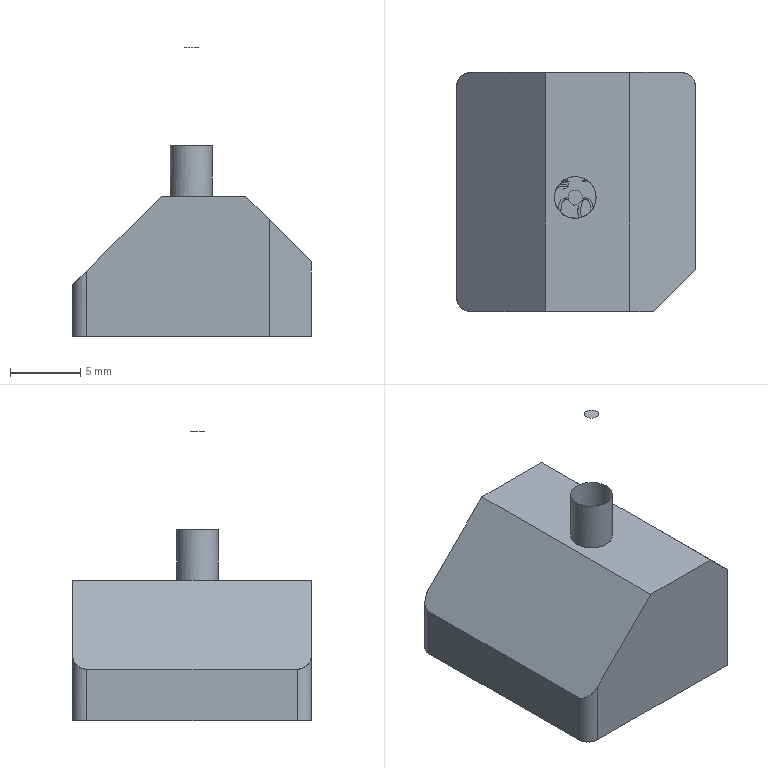NC program | PowerMill | posted with a generic post | part box 17 x 17 x 20.603 mm
Lines 3446 to 4194 of 69435:
N3543 M6
N3544 S8500 M03
N3545 G00 G90 X0.002 Y0.0
N3546 G43 Z11.803 H3
N3547
N3548 G05 P10000 R8
N3549 X2.657 Y10.5422
N3550 Z0.9529
N3551 G01 Z-0.2471 F360.0
N3552 X1.3839 Y5.4231 F600.0
N3553 X-4.833 Y-4.026
N3554 X-4.8208 Y-4.0426
N3555 G03 X-4.4372 Y-4.4965 I5.5114 J4.2692
N3556 G01 X-4.1788 Y-4.7566
N3557 X-3.8542 Y-5.0424
N3558 X-3.7339 Y-5.1386
N3559 X-3.531 Y-5.2892
N3560 X-3.2148 Y-5.4994
N3561 X-2.889 Y-5.6879
N3562 X-2.7291 Y-5.7704
N3563 X-2.5666 Y-5.8477
N3564 X-2.2505 Y-5.9835
N3565 X-2.023 Y-6.0667
N3566 X-1.726 Y-6.16
N3567 X-1.6019 Y-6.1971
N3568 X-1.4915 Y-6.2234
N3569 X4.7268 Y3.2278
N3570 G00 Z11.803
N3571 G05 P0
N3572 (---------------)
N3573 ( END TOOLPATH : 精公基准台01-平坦面平行-D10 )
N3574 (---------------)
N3575 ( START TOOLPATH : 精公基准台01-基准面偏置-D10 )
N3576 (---------------)
N3577 G00 X0.002 Y0.0 Z9.8029
N3578 G05 P10000 R8
N3579 X-11.42 Y14.0289
N3580 Z-9.6
N3581 G01 Z-10.8 F360.0
N3582 X-6.8515 Y11.3918 F600.0
N3583 X-6.3619 Y2.3433
N3584 X-6.2705 Y2.5538
N3585 X-6.1275 Y2.8375
N3586 X-5.9674 Y3.1213
N3587 X-5.7484 Y3.4657
N3588 X-5.5905 Y3.6888
N3589 X-5.3328 Y4.0166
N3590 X-5.1227 Y4.2563
N3591 X-4.9538 Y4.4336
N3592 X-4.7725 Y4.6109
N3593 X-4.5356 Y4.8238
N3594 X-4.2123 Y5.0848
N3595 X-3.993 Y5.2444
N3596 X-3.7737 Y5.3913
N3597 X-3.652 Y5.4675
N3598 X-3.3719 Y5.6304
N3599 X-3.0918 Y5.7767
N3600 X-2.6893 Y5.9588
N3601 X-2.5315 Y6.0219
N3602 X-2.2514 Y6.1232
N3603 X-1.9713 Y6.2112
N3604 X-1.6911 Y6.286
N3605 X-1.411 Y6.3486
N3606 X-1.1309 Y6.3989
N3607 X-0.8508 Y6.4376
N3608 X-0.5706 Y6.4644
N3609 X-0.2905 Y6.4797
N3610 X-0.0104 Y6.4838
N3611 X0.2697 Y6.4764
N3612 X0.5499 Y6.4574
N3613 X0.83 Y6.4271
N3614 X1.1101 Y6.385
N3615 X1.3903 Y6.3312
N3616 X1.6704 Y6.2649
N3617 X1.9505 Y6.186
N3618 X2.2306 Y6.0943
N3619 X2.5846 Y5.9588
N3620 X2.8278 Y5.8524
N3621 X3.071 Y5.7346
N3622 X3.3511 Y5.5835
N3623 X3.6687 Y5.3913
N3624 X3.9301 Y5.2148
N3625 X4.1915 Y5.0199
N3626 X4.4309 Y4.8238
N3627 X4.7518 Y4.5303
N3628 X5.0177 Y4.2563
N3629 X5.1677 Y4.0876
N3630 X5.312 Y3.914
N3631 X5.4857 Y3.6888
N3632 X5.6845 Y3.405
N3633 X5.8723 Y3.1049
N3634 X6.0267 Y2.8293
N3635 X6.1655 Y2.5538
N3636 X6.2927 Y2.27
N3637 X6.4325 Y1.9092
N3638 X6.5151 Y1.664
N3639 X6.5868 Y1.4188
N3640 X6.6582 Y1.135
N3641 X6.7167 Y0.8513
N3642 X6.7632 Y0.5675
N3643 X6.7974 Y0.2838
N3644 X6.8198 Y0.0
N3645 X6.8303 Y-0.2838
N3646 X6.8291 Y-0.5675
N3647 X6.8166 Y-0.8513
N3648 X6.7922 Y-1.135
N3649 X6.7556 Y-1.4188
N3650 X6.7072 Y-1.7025
N3651 X6.6462 Y-1.9863
N3652 X6.5728 Y-2.27
N3653 X6.4859 Y-2.5538
N3654 X6.4325 Y-2.7095
N3655 X6.2708 Y-3.1213
N3656 X6.141 Y-3.405
N3657 X5.9945 Y-3.6888
N3658 X5.8723 Y-3.9049
N3659 X5.6501 Y-4.2563
N3660 X5.4883 Y-4.4851
N3661 X5.312 Y-4.714
N3662 X5.222 Y-4.8238
N3663 X4.9987 Y-5.077
N3664 X4.6883 Y-5.3913
N3665 X4.4399 Y-5.6161
N3666 X4.1915 Y-5.8199
N3667 X4.0082 Y-5.9588
N3668 X3.6313 Y-6.2153
N3669 X3.3592 Y-6.379
N3670 X3.071 Y-6.5346
N3671 X2.7909 Y-6.6692
N3672 X2.5108 Y-6.7889
N3673 X2.2306 Y-6.8943
N3674 X1.9505 Y-6.986
N3675 X1.5541 Y-7.0938
N3676 X1.3903 Y-7.1312
N3677 X1.1101 Y-7.1849
N3678 X0.83 Y-7.227
N3679 X0.5499 Y-7.2576
N3680 X0.2697 Y-7.2764
N3681 X-0.0104 Y-7.2837
N3682 X-0.2905 Y-7.2797
N3683 X-0.5706 Y-7.2643
N3684 X-0.8508 Y-7.2376
N3685 X-1.1309 Y-7.1989
N3686 X-1.411 Y-7.1486
N3687 X-1.6588 Y-7.0938
N3688 X-1.9713 Y-7.0112
N3689 X-2.2514 Y-6.9233
N3690 X-2.5315 Y-6.8219
N3691 X-2.8116 Y-6.7068
N3692 X-3.0918 Y-6.5767
N3693 X-3.4219 Y-6.4028
N3694 X-3.652 Y-6.2674
N3695 X-3.8823 Y-6.1201
N3696 X-4.2123 Y-5.8848
N3697 X-4.4924 Y-5.6607
N3698 X-4.7725 Y-5.4109
N3699 X-5.0751 Y-5.1075
N3700 X-5.3267 Y-4.8238
N3701 X-5.5549 Y-4.5364
N3702 X-5.7549 Y-4.2563
N3703 X-5.893 Y-4.0426
N3704 X-6.0995 Y-3.6888
N3705 X-6.2457 Y-3.405
N3706 X-6.3756 Y-3.1213
N3707 X-6.4533 Y-2.9328
N3708 X-6.5906 Y-2.5538
N3709 X-6.6773 Y-2.27
N3710 X-6.7509 Y-1.9863
N3711 X-6.8119 Y-1.7025
N3712 X-6.8606 Y-1.4188
N3713 X-6.897 Y-1.135
N3714 X-6.9216 Y-0.8513
N3715 X-6.9337 Y-0.5675
N3716 X-6.935 Y-0.2838
N3717 X-6.9248 Y0.0
N3718 X-6.9022 Y0.2838
N3719 X-6.868 Y0.5675
N3720 X-6.8215 Y0.8513
N3721 X-6.7629 Y1.135
N3722 X-6.6918 Y1.4188
N3723 X-6.6073 Y1.7025
N3724 X-6.5093 Y1.9863
N3725 X-6.4533 Y2.1328
N3726 X-6.3619 Y2.3433
N3727 G00 Z9.8029
N3728 G05 P0
N3729 (---------------)
N3730 ( END TOOLPATH : 精公基准台01-基准面偏置-D10 )
N3731 (---------------)
N3732 ( START TOOLPATH : 精公基准台01-基准台侧光-D10 )
N3733 (---------------)
N3734 G00 X0.002 Y0.0 Z9.8029
N3735 G05 P10000 R8
N3736 X13.4804 Y-14.7765
N3737 Z-19.5
N3738 G01 Z-20.7 F360.0
N3739 G03 X9.9448 Y-11.241 I-1.7678 J1.7678 F600.0
N3740 G01 X9.1157 Y-12.0701
N3741 X9.1151 Y-12.0707
N3742 X9.1144 Y-12.0714
N3743 X8.9094 Y-12.2674
N3744 X8.908 Y-12.2686
N3745 X8.9066 Y-12.2699
N3746 X8.7687 Y-12.39
N3747 X8.7675 Y-12.3911
N3748 X8.7662 Y-12.3921
N3749 X8.588 Y-12.5349
N3750 X8.5863 Y-12.5362
N3751 X8.5846 Y-12.5375
N3752 X8.3433 Y-12.7108
N3753 X8.342 Y-12.7117
N3754 X8.3407 Y-12.7126
N3755 X8.2659 Y-12.762
N3756 X8.2644 Y-12.763
N3757 X8.2628 Y-12.764
N3758 X7.9467 Y-12.9528
N3759 X7.9448 Y-12.9539
N3760 X7.9429 Y-12.9549
N3761 X7.7951 Y-13.0328
N3762 X7.7939 Y-13.0334
N3763 X7.7926 Y-13.034
N3764 X7.6243 Y-13.1152
N3765 X7.6223 Y-13.1161
N3766 X7.6204 Y-13.117
N3767 X7.3042 Y-13.2494
N3768 X7.3018 Y-13.2503
N3769 X7.2993 Y-13.2512
N3770 X7.0005 Y-13.3538
N3771 X6.998 Y-13.3546
N3772 X6.9955 Y-13.3553
N3773 X6.662 Y-13.4457
N3774 X6.6594 Y-13.4463
N3775 X6.6568 Y-13.4469
N3776 X6.3406 Y-13.5102
N3777 X6.3381 Y-13.5107
N3778 X6.3356 Y-13.511
N3779 X6.0194 Y-13.5535
N3780 X6.0169 Y-13.5538
N3781 X6.0144 Y-13.554
N3782 X5.6982 Y-13.5762
N3783 X5.6959 Y-13.5763
N3784 X5.6935
N3785 X5.3774 Y-13.58
N3786 X5.3769
N3787 X5.3765
N3788 X-7.5855 Y-13.5793
N3789 X-7.5871 Y-13.5792
N3790 X-7.5887
N3791 X-7.9049 Y-13.5664
N3792 X-7.907 Y-13.5663
N3793 X-7.9091 Y-13.5661
N3794 X-8.2253 Y-13.5364
N3795 X-8.2274 Y-13.5361
N3796 X-8.2295 Y-13.5359
N3797 X-8.5456 Y-13.4891
N3798 X-8.5478 Y-13.4887
N3799 X-8.5498 Y-13.4883
N3800 X-8.866 Y-13.4242
N3801 X-8.8679 Y-13.4237
N3802 X-8.8699 Y-13.4233
N3803 X-9.1348 Y-13.3556
N3804 X-9.1369 Y-13.3551
N3805 X-9.139 Y-13.3544
N3806 X-9.5064 Y-13.2388
N3807 X-9.5087 Y-13.238
N3808 X-9.511 Y-13.2372
N3809 X-9.8271 Y-13.1162
N3810 X-9.8287 Y-13.1155
N3811 X-9.8304 Y-13.1148
N3812 X-10.0135 Y-13.0354
N3813 X-10.0146 Y-13.0349
N3814 X-10.0157 Y-13.0344
N3815 X-10.1487 Y-12.9719
N3816 X-10.1502 Y-12.9712
N3817 X-10.1517 Y-12.9704
N3818 X-10.4678 Y-12.8054
N3819 X-10.4694 Y-12.8046
N3820 X-10.4709 Y-12.8037
N3821 X-10.6239 Y-12.715
N3822 X-10.6249 Y-12.7144
N3823 X-10.6259 Y-12.7138
N3824 X-10.7892 Y-12.6124
N3825 X-10.7908 Y-12.6114
N3826 X-10.7924 Y-12.6103
N3827 X-11.1039 Y-12.3955
N3828 X-11.1061 Y-12.394
N3829 X-11.1081 Y-12.3924
N3830 X-11.4289 Y-12.1387
N3831 X-11.4302 Y-12.1376
N3832 X-11.4315 Y-12.1365
N3833 X-11.5039 Y-12.0741
N3834 X-11.505 Y-12.0732
N3835 X-11.506 Y-12.0722
N3836 X-11.7498 Y-11.8464
N3837 X-11.7509 Y-11.8454
N3838 X-11.752 Y-11.8443
N3839 X-11.8423 Y-11.754
N3840 X-11.8434 Y-11.7529
N3841 X-11.8444 Y-11.7518
N3842 X-12.0702 Y-11.508
N3843 X-12.0712 Y-11.507
N3844 X-12.0721 Y-11.5059
N3845 X-12.1346 Y-11.4335
N3846 X-12.1357 Y-11.4322
N3847 X-12.1367 Y-11.4309
N3848 X-12.3871 Y-11.1148
N3849 X-12.3887 Y-11.1127
N3850 X-12.3902 Y-11.1106
N3851 X-12.6085 Y-10.7944
N3852 X-12.6096 Y-10.7928
N3853 X-12.6106 Y-10.7912
N3854 X-12.7118 Y-10.6282
N3855 X-12.7124 Y-10.6272
N3856 X-12.713 Y-10.6262
N3857 X-12.8019 Y-10.4729
N3858 X-12.8028 Y-10.4714
N3859 X-12.8036 Y-10.4698
N3860 X-12.9687 Y-10.1537
N3861 X-12.9698 Y-10.1516
N3862 X-12.9708 Y-10.1494
N3863 X-13.1127 Y-9.8333
N3864 X-13.1136 Y-9.8312
N3865 X-13.1144 Y-9.8291
N3866 X-13.2354 Y-9.513
N3867 X-13.2361 Y-9.5109
N3868 X-13.2369 Y-9.5088
N3869 X-13.338 Y-9.1926
N3870 X-13.3387 Y-9.1905
N3871 X-13.3393 Y-9.1883
N3872 X-13.4213 Y-8.8722
N3873 X-13.4218 Y-8.8701
N3874 X-13.4223 Y-8.868
N3875 X-13.4867 Y-8.5519
N3876 X-13.4871 Y-8.5498
N3877 X-13.4875 Y-8.5476
N3878 X-13.5341 Y-8.2315
N3879 X-13.5344 Y-8.2294
N3880 X-13.5346 Y-8.2272
N3881 X-13.5642 Y-7.9111
N3882 X-13.5643 Y-7.909
N3883 X-13.5645 Y-7.907
N3884 X-13.5776 Y-7.5908
N3885 X-13.5777 Y-7.5892
N3886 Y-7.5875
N3887 Y0.0
N3888 Y7.5875
N3889 Y7.5892
N3890 X-13.5776 Y7.5908
N3891 X-13.5645 Y7.907
N3892 X-13.5643 Y7.909
N3893 X-13.5642 Y7.9111
N3894 X-13.5346 Y8.2272
N3895 X-13.5344 Y8.2294
N3896 X-13.5341 Y8.2315
N3897 X-13.4875 Y8.5476
N3898 X-13.4871 Y8.5498
N3899 X-13.4867 Y8.5519
N3900 X-13.4223 Y8.868
N3901 X-13.4219 Y8.8699
N3902 X-13.4214 Y8.8718
N3903 X-13.3536 Y9.1379
N3904 X-13.3531 Y9.14
N3905 X-13.3524 Y9.1422
N3906 X-13.237 Y9.5084
N3907 X-13.2362 Y9.5107
N3908 X-13.2354 Y9.513
N3909 X-13.1144 Y9.8291
N3910 X-13.1136 Y9.8312
N3911 X-13.1127 Y9.8333
N3912 X-12.9708 Y10.1494
N3913 X-12.9698 Y10.1516
N3914 X-12.9687 Y10.1537
N3915 X-12.8036 Y10.4698
N3916 X-12.8028 Y10.4714
N3917 X-12.8019 Y10.4729
N3918 X-12.713 Y10.6262
N3919 X-12.7124 Y10.6272
N3920 X-12.7118 Y10.6282
N3921 X-12.6106 Y10.7912
N3922 X-12.6096 Y10.7928
N3923 X-12.6085 Y10.7944
N3924 X-12.3935 Y11.106
N3925 X-12.392 Y11.1082
N3926 X-12.3904 Y11.1103
N3927 X-12.1367 Y11.4309
N3928 X-12.1357 Y11.4322
N3929 X-12.1346 Y11.4335
N3930 X-12.0721 Y11.5059
N3931 X-12.0712 Y11.507
N3932 X-12.0702 Y11.508
N3933 X-11.8444 Y11.7518
N3934 X-11.8434 Y11.7529
N3935 X-11.8423 Y11.754
N3936 X-11.752 Y11.8443
N3937 X-11.7509 Y11.8454
N3938 X-11.7498 Y11.8464
N3939 X-11.506 Y12.0722
N3940 X-11.505 Y12.0732
N3941 X-11.5039 Y12.0741
N3942 X-11.4315 Y12.1365
N3943 X-11.4302 Y12.1376
N3944 X-11.4289 Y12.1387
N3945 X-11.1128 Y12.389
N3946 X-11.1107 Y12.3906
N3947 X-11.1085 Y12.3921
N3948 X-10.7924 Y12.6103
N3949 X-10.7908 Y12.6114
N3950 X-10.7892 Y12.6124
N3951 X-10.6259 Y12.7138
N3952 X-10.6249 Y12.7144
N3953 X-10.6239 Y12.715
N3954 X-10.4709 Y12.8037
N3955 X-10.4694 Y12.8046
N3956 X-10.4678 Y12.8054
N3957 X-10.1517 Y12.9704
N3958 X-10.1502 Y12.9712
N3959 X-10.1487 Y12.9719
N3960 X-10.0157 Y13.0344
N3961 X-10.0146 Y13.0349
N3962 X-10.0135 Y13.0354
N3963 X-9.8304 Y13.1148
N3964 X-9.8287 Y13.1155
N3965 X-9.8271 Y13.1162
N3966 X-9.511 Y13.2372
N3967 X-9.5089 Y13.2379
N3968 X-9.5067 Y13.2387
N3969 X-9.1906 Y13.3397
N3970 X-9.1885 Y13.3404
N3971 X-9.1864 Y13.341
N3972 X-8.8702 Y13.4232
N3973 X-8.8681 Y13.4237
N3974 X-8.866 Y13.4242
N3975 X-8.5498 Y13.4883
N3976 X-8.5477 Y13.4887
N3977 X-8.5456 Y13.4891
N3978 X-8.2295 Y13.5359
N3979 X-8.2274 Y13.5361
N3980 X-8.2253 Y13.5364
N3981 X-7.9091 Y13.5661
N3982 X-7.907 Y13.5663
N3983 X-7.9049 Y13.5664
N3984 X-7.5887 Y13.5792
N3985 X-7.5871
N3986 X-7.5855 Y13.5793
N3987 X0.002 Y13.5792
N3988 X7.5895
N3989 X7.5912
N3990 X7.5928
N3991 X7.909 Y13.566
N3992 X7.911 Y13.5659
N3993 X7.9131 Y13.5657
N3994 X8.2292 Y13.5362
N3995 X8.2314 Y13.536
N3996 X8.2335 Y13.5357
N3997 X8.5496 Y13.4889
N3998 X8.5518 Y13.4886
N3999 X8.554 Y13.4881
N4000 X8.8702 Y13.4232
N4001 X8.8719 Y13.4228
N4002 X8.8737 Y13.4224
N4003 X9.1377 Y13.3557
N4004 X9.14 Y13.3551
N4005 X9.1423 Y13.3544
N4006 X9.5105 Y13.2378
N4007 X9.5127 Y13.2371
N4008 X9.5148 Y13.2363
N4009 X9.831 Y13.116
N4010 X9.8332 Y13.1152
N4011 X9.8353 Y13.1142
N4012 X10.1515 Y12.972
N4013 X10.1536 Y12.9711
N4014 X10.1557 Y12.97
N4015 X10.4718 Y12.8049
N4016 X10.4734 Y12.8041
N4017 X10.4749 Y12.8032
N4018 X10.627 Y12.715
N4019 X10.6281 Y12.7144
N4020 X10.6291 Y12.7138
N4021 X10.7932 Y12.6119
N4022 X10.7948 Y12.6109
N4023 X10.7964 Y12.6098
N4024 X11.1069 Y12.3955
N4025 X11.1091 Y12.394
N4026 X11.1112 Y12.3924
N4027 X11.4329 Y12.1376
N4028 X11.4342 Y12.1365
N4029 X11.4354 Y12.1355
N4030 X11.5066 Y12.0742
N4031 X11.5077 Y12.0732
N4032 X11.5088 Y12.0723
N4033 X11.7537 Y11.8456
N4034 X11.7549 Y11.8446
N4035 X11.756 Y11.8435
N4036 X11.8455 Y11.754
N4037 X11.8466 Y11.7528
N4038 X11.8476 Y11.7517
N4039 X12.0743 Y11.5067
N4040 X12.0752 Y11.5057
N4041 X12.0762 Y11.5046
N4042 X12.1374 Y11.4334
N4043 X12.1385 Y11.4322
N4044 X12.1395 Y11.4309
N4045 X12.3902 Y11.1148
N4046 X12.3918 Y11.1127
N4047 X12.3933 Y11.1106
N4048 X12.6116 Y10.7944
N4049 X12.6127 Y10.7928
N4050 X12.6137 Y10.7912
N4051 X12.7158 Y10.6268
N4052 X12.7164 Y10.6258
N4053 X12.717 Y10.6247
N4054 X12.8051 Y10.4729
N4055 X12.8059 Y10.4714
N4056 X12.8068 Y10.4698
N4057 X12.9718 Y10.1537
N4058 X12.9728 Y10.1516
N4059 X12.9738 Y10.1495
N4060 X13.116 Y9.8333
N4061 X13.1169 Y9.8312
N4062 X13.1178 Y9.829
N4063 X13.238 Y9.5128
N4064 X13.2388 Y9.5109
N4065 X13.2394 Y9.5089
N4066 X13.3412 Y9.1927
N4067 X13.3418 Y9.1905
N4068 X13.3425 Y9.1882
N4069 X13.424 Y8.8721
N4070 X13.4245 Y8.8701
N4071 X13.4249 Y8.8682
N4072 X13.4898 Y8.552
N4073 X13.4902 Y8.5498
N4074 X13.4906 Y8.5476
N4075 X13.5373 Y8.2315
N4076 X13.5376 Y8.2294
N4077 X13.5378 Y8.2272
N4078 X13.5673 Y7.9111
N4079 X13.5675 Y7.909
N4080 X13.5676 Y7.907
N4081 X13.5808 Y7.5908
N4082 Y7.5892
N4083 Y7.5875
N4084 X13.5816 Y-5.3745
N4085 Y-5.3749
N4086 Y-5.3754
N4087 X13.5779 Y-5.6915
N4088 Y-5.6939
N4089 X13.5778 Y-5.6962
N4090 X13.5556 Y-6.0124
N4091 X13.5554 Y-6.0149
N4092 X13.5551 Y-6.0174
N4093 X13.5127 Y-6.3336
N4094 X13.5123 Y-6.3361
N4095 X13.5118 Y-6.3386
N4096 X13.4486 Y-6.6548
N4097 X13.448 Y-6.6573
N4098 X13.4474 Y-6.6598
N4099 X13.3624 Y-6.976
N4100 X13.3617 Y-6.9785
N4101 X13.3608 Y-6.981
N4102 X13.253 Y-7.2972
N4103 X13.2521 Y-7.2997
N4104 X13.2511 Y-7.3022
N4105 X13.1188 Y-7.6184
N4106 X13.1179 Y-7.6203
N4107 X13.117 Y-7.6222
N4108 X13.036 Y-7.7902
N4109 X13.0354 Y-7.7915
N4110 X13.0348 Y-7.7927
N4111 X12.9567 Y-7.9409
N4112 X12.9557 Y-7.9428
N4113 X12.9546 Y-7.9447
N4114 X12.7658 Y-8.2608
N4115 X12.7649 Y-8.2624
N4116 X12.7639 Y-8.2639
N4117 X12.7146 Y-8.3385
N4118 X12.7137 Y-8.3398
N4119 X12.7128 Y-8.3411
N4120 X12.5394 Y-8.5826
N4121 X12.5381 Y-8.5843
N4122 X12.5368 Y-8.5859
N4123 X12.3941 Y-8.7641
N4124 X12.3931 Y-8.7654
N4125 X12.392 Y-8.7666
N4126 X12.2718 Y-8.9046
N4127 X12.2706 Y-8.906
N4128 X12.2693 Y-8.9074
N4129 X12.0734 Y-9.1124
N4130 X12.0727 Y-9.113
N4131 X12.0721 Y-9.1137
N4132 X9.9448 Y-11.241
N4133 G03 X13.4804 Y-14.7765 I1.7678 J-1.7677
N4134 G01 X13.4289 Y-14.7148
N4135 G03 X9.8934 Y-11.1793 I-1.7677 J1.7678
N4136 G01 X9.0591 Y-12.0135
N4137 X8.8541 Y-12.2095
N4138 X8.7162 Y-12.3297
N4139 X8.5379 Y-12.4725
N4140 X8.2966 Y-12.6458
N4141 X8.2218 Y-12.6953
N4142 X7.9056 Y-12.8841
N4143 X7.7579 Y-12.962
N4144 X7.5895 Y-13.0432
N4145 X7.2734 Y-13.1756
N4146 X6.9745 Y-13.2781
N4147 X6.6411 Y-13.3684
N4148 X6.3249 Y-13.4318
N4149 X6.0088 Y-13.4742
N4150 X5.6926 Y-13.4964
N4151 X5.3765 Y-13.5
N4152 X-7.2694
N4153 X-7.5855 Y-13.4993
N4154 X-7.9016 Y-13.4864
N4155 X-8.2178 Y-13.4567
N4156 X-8.5339 Y-13.4099
N4157 X-8.8501 Y-13.3458
N4158 X-9.115 Y-13.2781
N4159 X-9.4824 Y-13.1625
N4160 X-9.7985 Y-13.0415
N4161 X-9.9817 Y-12.962
N4162 X-10.1147 Y-12.8995
N4163 X-10.4308 Y-12.7345
N4164 X-10.5837 Y-12.6458
N4165 X-10.747 Y-12.5445
N4166 X-11.0585 Y-12.3297
N4167 X-11.3792 Y-12.0759
N4168 X-11.4517 Y-12.0135
N4169 X-11.6954 Y-11.7877
N4170 X-11.7857 Y-11.6974
N4171 X-12.0115 Y-11.4537
N4172 X-12.074 Y-11.3812
N4173 X-12.3244 Y-11.0651
N4174 X-12.5427 Y-10.749
N4175 X-12.6438 Y-10.586
N4176 X-12.7327 Y-10.4328
N4177 X-12.8978 Y-10.1167
N4178 X-13.0397 Y-9.8005
N4179 X-13.1607 Y-9.4844
N4180 X-13.2619 Y-9.1682
N4181 X-13.3439 Y-8.8521
N4182 X-13.4083 Y-8.5359
N4183 X-13.455 Y-8.2198
N4184 X-13.4845 Y-7.9036
N4185 X-13.4977 Y-7.5875
N4186 X-13.4984 Y-7.2714
N4187 Y0.0
N4188 Y7.2714
N4189 X-13.4977 Y7.5875
N4190 X-13.4845 Y7.9036
N4191 X-13.455 Y8.2198
N4192 X-13.4083 Y8.5359
N4193 X-13.3439 Y8.8521
N4194 X-13.2761 Y9.1181
N4195 X-13.1607 Y9.4844
N4196 X-13.0397 Y9.8005
N4197 X-12.8978 Y10.1167
N4198 X-12.7327 Y10.4328
N4199 X-12.6438 Y10.586
N4200 X-12.5427 Y10.749
N4201 X-12.3277 Y11.0606
N4202 X-12.074 Y11.3812
N4203 X-12.0115 Y11.4537
N4204 X-11.7857 Y11.6974
N4205 X-11.6954 Y11.7877
N4206 X-11.4517 Y12.0135
N4207 X-11.3792 Y12.0759
N4208 X-11.0631 Y12.3263
N4209 X-10.747 Y12.5445
N4210 X-10.5837 Y12.6458
N4211 X-10.4308 Y12.7345
N4212 X-10.1147 Y12.8995
N4213 X-9.9817 Y12.962
N4214 X-9.7985 Y13.0414
N4215 X-9.4824 Y13.1625
N4216 X-9.1662 Y13.2635
N4217 X-8.8501 Y13.3458
N4218 X-8.5339 Y13.4099
N4219 X-8.2178 Y13.4567
N4220 X-7.9016 Y13.4864
N4221 X-7.5855 Y13.4993
N4222 X-7.2694 Y13.5
N4223 X0.002
N4224 X7.2734
N4225 X7.5895 Y13.4992
N4226 X7.9056 Y13.4861
N4227 X8.2218 Y13.4566
N4228 X8.5379 Y13.4098
N4229 X8.8541 Y13.3449
N4230 X9.1181 Y13.2781
N4231 X9.4864 Y13.1616
N4232 X9.8025 Y13.0413
N4233 X10.1187 Y12.8991
N4234 X10.4348 Y12.734
N4235 X10.5869 Y12.6458
N4236 X10.751 Y12.5439
N4237 X11.0615 Y12.3297
N4238 X11.3832 Y12.0749
N4239 X11.4544 Y12.0135
N4240 X11.6994 Y11.7869
N4241 X11.7889 Y11.6974
N4242 X12.0155 Y11.4524
N4243 X12.0768 Y11.3812
N4244 X12.3275 Y11.0651
N4245 X12.5458 Y10.749
N4246 X12.6478 Y10.5846
N4247 X12.7358 Y10.4328
N4248 X12.9009 Y10.1167
N4249 X13.043 Y9.8005
N4250 X13.1633 Y9.4844
N4251 X13.265 Y9.1682
N4252 X13.3465 Y8.8521
N4253 X13.4114 Y8.5359
N4254 X13.4582 Y8.2198
N4255 X13.4877 Y7.9036
N4256 X13.5008 Y7.5875
N4257 X13.5016 Y7.2714
N4258 Y-5.3745
N4259 X13.498 Y-5.6906
N4260 X13.4758 Y-6.0068
N4261 X13.4334 Y-6.3229
N4262 X13.3701 Y-6.6391
N4263 X13.2851 Y-6.9552
N4264 X13.1773 Y-7.2714
N4265 X13.045 Y-7.5875
N4266 X12.964 Y-7.7555
N4267 X12.8859 Y-7.9036
N4268 X12.6972 Y-8.2198
N4269 X12.6478 Y-8.2944
N4270 X12.4744 Y-8.5359
N4271 X12.3317 Y-8.7141
N4272 X12.2115 Y-8.8521
N4273 X12.0155 Y-9.0571
N4274 X9.8934 Y-11.1793
N4275 G03 X13.4289 Y-14.7148 I1.7678 J-1.7677
N4276 G00 Z9.8029
N4277 G05 P0
N4278 (---------------)
N4279 ( END TOOLPATH : 精公基准台01-基准台侧光-D10 )
N4280 (---------------)
N4281
N4282 M05
N4283 G53 Z0.0
N4284 (---------------)
N4285 ( START TOOLPATH : 精公精光01-等高-D4 )
N4286 (---------------)
N4287 ( TOOL NO.    :14 )
N4288 ( TOOL TYPE   : ENDMILL)
N4289 ( TOOL ID     : D4_1_1)
N4290 ( TOOL DIA    : 4.0 LENGTH 65.76)
N4291 T14